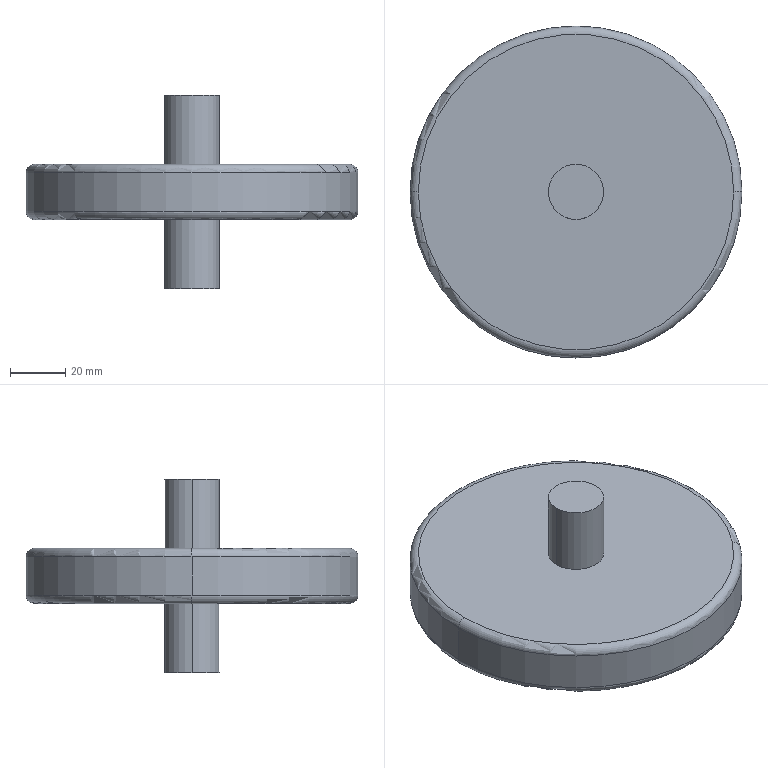Part | SolidWorks | features ICE 2, Extrusion 1, Fillet 1 | 1 solid | 14 faces | box 120 x 120 x 70 mm | volume 240463 mm3 | cylinder 6 | torus 4 | plane 4 | commonest cylinder face diameters 20 x4 120 x2
STEP:
#1=CARTESIAN_POINT('',(10.,0.,45.));
#2=VERTEX_POINT('',#1);
#3=CARTESIAN_POINT('',(-10.,0.,45.));
#4=VERTEX_POINT('',#3);
#5=CARTESIAN_POINT('',(0.,0.,45.));
#6=DIRECTION('',(0.,0.,1.));
#7=DIRECTION('',(1.,0.,0.));
#8=AXIS2_PLACEMENT_3D('',#5,#6,#7);
#9=CIRCLE('',#8,10.);
#10=EDGE_CURVE('',#2,#4,#9,.T.);
#11=ORIENTED_EDGE('',*,*,#10,.F.);
#12=CARTESIAN_POINT('',(10.,0.,20.));
#13=VERTEX_POINT('',#12);
#14=CARTESIAN_POINT('',(10.,0.,45.));
#15=DIRECTION('',(0.,0.,-1.));
#16=VECTOR('',#15,1000.);
#17=LINE('',#14,#16);
#18=EDGE_CURVE('',#2,#13,#17,.T.);
#19=ORIENTED_EDGE('',*,*,#18,.T.);
#20=CARTESIAN_POINT('',(-10.,0.,20.));
#21=VERTEX_POINT('',#20);
#22=CARTESIAN_POINT('',(0.,0.,20.));
#23=DIRECTION('',(0.,0.,1.));
#24=DIRECTION('',(1.,0.,0.));
#25=AXIS2_PLACEMENT_3D('',#22,#23,#24);
#26=CIRCLE('',#25,10.);
#27=EDGE_CURVE('',#13,#21,#26,.T.);
#28=ORIENTED_EDGE('',*,*,#27,.T.);
#29=CARTESIAN_POINT('',(-10.,0.,45.));
#30=DIRECTION('',(0.,0.,-1.));
#31=VECTOR('',#30,1000.);
#32=LINE('',#29,#31);
#33=EDGE_CURVE('',#4,#21,#32,.T.);
#34=ORIENTED_EDGE('',*,*,#33,.F.);
#35=EDGE_LOOP('',(#11,#19,#28,#34));
#36=FACE_OUTER_BOUND('',#35,.T.);
#37=CARTESIAN_POINT('',(0.,0.,45.));
#38=DIRECTION('',(0.,0.,-1.));
#39=DIRECTION('',(-1.,0.,0.));
#40=AXIS2_PLACEMENT_3D('',#37,#38,#39);
#41=CYLINDRICAL_SURFACE('',#40,10.);
#42=ADVANCED_FACE('',(#36),#41,.T.);
#43=CARTESIAN_POINT('',(-10.,0.,-25.));
#44=VERTEX_POINT('',#43);
#45=CARTESIAN_POINT('',(10.,0.,-25.));
#46=VERTEX_POINT('',#45);
#47=CARTESIAN_POINT('',(0.,0.,-25.));
#48=DIRECTION('',(0.,0.,-1.));
#49=DIRECTION('',(-1.,0.,0.));
#50=AXIS2_PLACEMENT_3D('',#47,#48,#49);
#51=CIRCLE('',#50,10.);
#52=EDGE_CURVE('',#44,#46,#51,.T.);
#53=ORIENTED_EDGE('',*,*,#52,.F.);
#54=CARTESIAN_POINT('',(-10.,0.,0.));
#55=VERTEX_POINT('',#54);
#56=CARTESIAN_POINT('',(-10.,0.,-25.));
#57=DIRECTION('',(0.,0.,1.));
#58=VECTOR('',#57,1000.);
#59=LINE('',#56,#58);
#60=EDGE_CURVE('',#44,#55,#59,.T.);
#61=ORIENTED_EDGE('',*,*,#60,.T.);
#62=CARTESIAN_POINT('',(10.,0.,0.));
#63=VERTEX_POINT('',#62);
#64=CARTESIAN_POINT('',(0.,0.,0.));
#65=DIRECTION('',(0.,0.,-1.));
#66=DIRECTION('',(1.,0.,0.));
#67=AXIS2_PLACEMENT_3D('',#64,#65,#66);
#68=CIRCLE('',#67,10.);
#69=EDGE_CURVE('',#55,#63,#68,.T.);
#70=ORIENTED_EDGE('',*,*,#69,.T.);
#71=CARTESIAN_POINT('',(10.,0.,-25.));
#72=DIRECTION('',(0.,0.,1.));
#73=VECTOR('',#72,1000.);
#74=LINE('',#71,#73);
#75=EDGE_CURVE('',#46,#63,#74,.T.);
#76=ORIENTED_EDGE('',*,*,#75,.F.);
#77=EDGE_LOOP('',(#53,#61,#70,#76));
#78=FACE_OUTER_BOUND('',#77,.T.);
#79=CARTESIAN_POINT('',(0.,0.,-25.));
#80=DIRECTION('',(0.,0.,1.));
#81=DIRECTION('',(1.,0.,0.));
#82=AXIS2_PLACEMENT_3D('',#79,#80,#81);
#83=CYLINDRICAL_SURFACE('',#82,10.);
#84=ADVANCED_FACE('',(#78),#83,.T.);
#85=CARTESIAN_POINT('',(-60.,0.,17.));
#86=VERTEX_POINT('',#85);
#87=CARTESIAN_POINT('',(60.,0.,17.));
#88=VERTEX_POINT('',#87);
#89=CARTESIAN_POINT('',(0.,0.,17.));
#90=DIRECTION('',(0.,0.,-1.));
#91=DIRECTION('',(1.,0.,0.));
#92=AXIS2_PLACEMENT_3D('',#89,#90,#91);
#93=CIRCLE('',#92,60.);
#94=EDGE_CURVE('',#86,#88,#93,.T.);
#95=ORIENTED_EDGE('',*,*,#94,.F.);
#96=CARTESIAN_POINT('',(-57.,0.,20.));
#97=VERTEX_POINT('',#96);
#98=CARTESIAN_POINT('',(-57.,0.,17.));
#99=DIRECTION('',(0.,1.,0.));
#100=DIRECTION('',(-1.,0.,0.));
#101=AXIS2_PLACEMENT_3D('',#98,#99,#100);
#102=CIRCLE('',#101,3.);
#103=EDGE_CURVE('',#86,#97,#102,.T.);
#104=ORIENTED_EDGE('',*,*,#103,.T.);
#105=CARTESIAN_POINT('',(57.,0.,20.));
#106=VERTEX_POINT('',#105);
#107=CARTESIAN_POINT('',(0.,0.,20.));
#108=DIRECTION('',(0.,0.,1.));
#109=DIRECTION('',(1.,0.,0.));
#110=AXIS2_PLACEMENT_3D('',#107,#108,#109);
#111=CIRCLE('',#110,57.);
#112=EDGE_CURVE('',#106,#97,#111,.T.);
#113=ORIENTED_EDGE('',*,*,#112,.F.);
#114=CARTESIAN_POINT('',(57.,0.,17.));
#115=DIRECTION('',(0.,-1.,0.));
#116=DIRECTION('',(0.,0.,-1.));
#117=AXIS2_PLACEMENT_3D('',#114,#115,#116);
#118=CIRCLE('',#117,3.);
#119=EDGE_CURVE('',#88,#106,#118,.T.);
#120=ORIENTED_EDGE('',*,*,#119,.F.);
#121=EDGE_LOOP('',(#95,#104,#113,#120));
#122=FACE_OUTER_BOUND('',#121,.T.);
#123=CARTESIAN_POINT('',(0.,0.,17.));
#124=DIRECTION('',(0.,0.,1.));
#125=DIRECTION('',(1.,0.,0.));
#126=AXIS2_PLACEMENT_3D('',#123,#124,#125);
#127=TOROIDAL_SURFACE('',#126,57.,3.);
#128=ADVANCED_FACE('',(#122),#127,.T.);
#129=CARTESIAN_POINT('',(-57.,0.,0.));
#130=VERTEX_POINT('',#129);
#131=CARTESIAN_POINT('',(57.,0.,0.));
#132=VERTEX_POINT('',#131);
#133=CARTESIAN_POINT('',(0.,0.,0.));
#134=DIRECTION('',(0.,0.,-1.));
#135=DIRECTION('',(1.,0.,0.));
#136=AXIS2_PLACEMENT_3D('',#133,#134,#135);
#137=CIRCLE('',#136,57.);
#138=EDGE_CURVE('',#130,#132,#137,.T.);
#139=ORIENTED_EDGE('',*,*,#138,.F.);
#140=CARTESIAN_POINT('',(-60.,0.,3.));
#141=VERTEX_POINT('',#140);
#142=CARTESIAN_POINT('',(-57.,0.,3.));
#143=DIRECTION('',(0.,1.,0.));
#144=DIRECTION('',(-1.,0.,0.));
#145=AXIS2_PLACEMENT_3D('',#142,#143,#144);
#146=CIRCLE('',#145,3.);
#147=EDGE_CURVE('',#130,#141,#146,.T.);
#148=ORIENTED_EDGE('',*,*,#147,.T.);
#149=CARTESIAN_POINT('',(60.,0.,3.));
#150=VERTEX_POINT('',#149);
#151=CARTESIAN_POINT('',(0.,0.,3.));
#152=DIRECTION('',(0.,0.,1.));
#153=DIRECTION('',(1.,0.,0.));
#154=AXIS2_PLACEMENT_3D('',#151,#152,#153);
#155=CIRCLE('',#154,60.);
#156=EDGE_CURVE('',#150,#141,#155,.T.);
#157=ORIENTED_EDGE('',*,*,#156,.F.);
#158=CARTESIAN_POINT('',(57.,0.,3.));
#159=DIRECTION('',(0.,-1.,0.));
#160=DIRECTION('',(0.,0.,-1.));
#161=AXIS2_PLACEMENT_3D('',#158,#159,#160);
#162=CIRCLE('',#161,3.);
#163=EDGE_CURVE('',#132,#150,#162,.T.);
#164=ORIENTED_EDGE('',*,*,#163,.F.);
#165=EDGE_LOOP('',(#139,#148,#157,#164));
#166=FACE_OUTER_BOUND('',#165,.T.);
#167=CARTESIAN_POINT('',(0.,0.,3.));
#168=DIRECTION('',(0.,0.,1.));
#169=DIRECTION('',(1.,0.,0.));
#170=AXIS2_PLACEMENT_3D('',#167,#168,#169);
#171=TOROIDAL_SURFACE('',#170,57.,3.);
#172=ADVANCED_FACE('',(#166),#171,.T.);
#173=ORIENTED_EDGE('',*,*,#94,.T.);
#174=CARTESIAN_POINT('',(60.,0.,20.));
#175=DIRECTION('',(0.,0.,-1.));
#176=VECTOR('',#175,1000.);
#177=LINE('',#174,#176);
#178=EDGE_CURVE('',#88,#150,#177,.T.);
#179=ORIENTED_EDGE('',*,*,#178,.T.);
#180=ORIENTED_EDGE('',*,*,#156,.T.);
#181=CARTESIAN_POINT('',(-60.,0.,20.));
#182=DIRECTION('',(0.,0.,-1.));
#183=VECTOR('',#182,1000.);
#184=LINE('',#181,#183);
#185=EDGE_CURVE('',#86,#141,#184,.T.);
#186=ORIENTED_EDGE('',*,*,#185,.F.);
#187=EDGE_LOOP('',(#173,#179,#180,#186));
#188=FACE_OUTER_BOUND('',#187,.T.);
#189=CARTESIAN_POINT('',(0.,0.,20.));
#190=DIRECTION('',(0.,0.,-1.));
#191=DIRECTION('',(-1.,0.,0.));
#192=AXIS2_PLACEMENT_3D('',#189,#190,#191);
#193=CYLINDRICAL_SURFACE('',#192,60.);
#194=ADVANCED_FACE('',(#188),#193,.T.);
#195=ORIENTED_EDGE('',*,*,#178,.F.);
#196=CARTESIAN_POINT('',(0.,0.,17.));
#197=DIRECTION('',(0.,0.,-1.));
#198=DIRECTION('',(1.,0.,0.));
#199=AXIS2_PLACEMENT_3D('',#196,#197,#198);
#200=CIRCLE('',#199,60.);
#201=EDGE_CURVE('',#88,#86,#200,.T.);
#202=ORIENTED_EDGE('',*,*,#201,.T.);
#203=ORIENTED_EDGE('',*,*,#185,.T.);
#204=CARTESIAN_POINT('',(0.,0.,3.));
#205=DIRECTION('',(0.,0.,1.));
#206=DIRECTION('',(1.,0.,0.));
#207=AXIS2_PLACEMENT_3D('',#204,#205,#206);
#208=CIRCLE('',#207,60.);
#209=EDGE_CURVE('',#141,#150,#208,.T.);
#210=ORIENTED_EDGE('',*,*,#209,.T.);
#211=EDGE_LOOP('',(#195,#202,#203,#210));
#212=FACE_OUTER_BOUND('',#211,.T.);
#213=CARTESIAN_POINT('',(0.,0.,20.));
#214=DIRECTION('',(0.,0.,-1.));
#215=DIRECTION('',(-1.,0.,0.));
#216=AXIS2_PLACEMENT_3D('',#213,#214,#215);
#217=CYLINDRICAL_SURFACE('',#216,60.);
#218=ADVANCED_FACE('',(#212),#217,.T.);
#219=CARTESIAN_POINT('',(0.,0.,20.));
#220=DIRECTION('',(0.,0.,1.));
#221=DIRECTION('',(1.,0.,0.));
#222=AXIS2_PLACEMENT_3D('',#219,#220,#221);
#223=CIRCLE('',#222,10.);
#224=EDGE_CURVE('',#21,#13,#223,.T.);
#225=ORIENTED_EDGE('',*,*,#224,.F.);
#226=ORIENTED_EDGE('',*,*,#27,.F.);
#227=EDGE_LOOP('',(#225,#226));
#228=FACE_BOUND('',#227,.T.);
#229=ORIENTED_EDGE('',*,*,#112,.T.);
#230=CARTESIAN_POINT('',(0.,0.,20.));
#231=DIRECTION('',(0.,0.,1.));
#232=DIRECTION('',(1.,0.,0.));
#233=AXIS2_PLACEMENT_3D('',#230,#231,#232);
#234=CIRCLE('',#233,57.);
#235=EDGE_CURVE('',#97,#106,#234,.T.);
#236=ORIENTED_EDGE('',*,*,#235,.T.);
#237=EDGE_LOOP('',(#229,#236));
#238=FACE_OUTER_BOUND('',#237,.T.);
#239=CARTESIAN_POINT('',(0.,0.,20.));
#240=DIRECTION('',(0.,0.,1.));
#241=DIRECTION('',(1.,0.,0.));
#242=AXIS2_PLACEMENT_3D('',#239,#240,#241);
#243=PLANE('',#242);
#244=ADVANCED_FACE('',(#228,#238),#243,.T.);
#245=CARTESIAN_POINT('',(0.,0.,0.));
#246=DIRECTION('',(0.,0.,-1.));
#247=DIRECTION('',(1.,0.,0.));
#248=AXIS2_PLACEMENT_3D('',#245,#246,#247);
#249=CIRCLE('',#248,10.);
#250=EDGE_CURVE('',#63,#55,#249,.T.);
#251=ORIENTED_EDGE('',*,*,#250,.F.);
#252=ORIENTED_EDGE('',*,*,#69,.F.);
#253=EDGE_LOOP('',(#251,#252));
#254=FACE_BOUND('',#253,.T.);
#255=CARTESIAN_POINT('',(0.,0.,0.));
#256=DIRECTION('',(0.,0.,-1.));
#257=DIRECTION('',(1.,0.,0.));
#258=AXIS2_PLACEMENT_3D('',#255,#256,#257);
#259=CIRCLE('',#258,57.);
#260=EDGE_CURVE('',#132,#130,#259,.T.);
#261=ORIENTED_EDGE('',*,*,#260,.T.);
#262=ORIENTED_EDGE('',*,*,#138,.T.);
#263=EDGE_LOOP('',(#261,#262));
#264=FACE_OUTER_BOUND('',#263,.T.);
#265=CARTESIAN_POINT('',(0.,0.,0.));
#266=DIRECTION('',(0.,0.,1.));
#267=DIRECTION('',(1.,0.,0.));
#268=AXIS2_PLACEMENT_3D('',#265,#266,#267);
#269=PLANE('',#268);
#270=ADVANCED_FACE('',(#254,#264),#269,.F.);
#271=ORIENTED_EDGE('',*,*,#147,.F.);
#272=ORIENTED_EDGE('',*,*,#260,.F.);
#273=ORIENTED_EDGE('',*,*,#163,.T.);
#274=ORIENTED_EDGE('',*,*,#209,.F.);
#275=EDGE_LOOP('',(#271,#272,#273,#274));
#276=FACE_OUTER_BOUND('',#275,.T.);
#277=CARTESIAN_POINT('',(0.,0.,3.));
#278=DIRECTION('',(0.,0.,1.));
#279=DIRECTION('',(1.,0.,0.));
#280=AXIS2_PLACEMENT_3D('',#277,#278,#279);
#281=TOROIDAL_SURFACE('',#280,57.,3.);
#282=ADVANCED_FACE('',(#276),#281,.T.);
#283=ORIENTED_EDGE('',*,*,#103,.F.);
#284=ORIENTED_EDGE('',*,*,#201,.F.);
#285=ORIENTED_EDGE('',*,*,#119,.T.);
#286=ORIENTED_EDGE('',*,*,#235,.F.);
#287=EDGE_LOOP('',(#283,#284,#285,#286));
#288=FACE_OUTER_BOUND('',#287,.T.);
#289=CARTESIAN_POINT('',(0.,0.,17.));
#290=DIRECTION('',(0.,0.,1.));
#291=DIRECTION('',(1.,0.,0.));
#292=AXIS2_PLACEMENT_3D('',#289,#290,#291);
#293=TOROIDAL_SURFACE('',#292,57.,3.);
#294=ADVANCED_FACE('',(#288),#293,.T.);
#295=ORIENTED_EDGE('',*,*,#60,.F.);
#296=CARTESIAN_POINT('',(0.,0.,-25.));
#297=DIRECTION('',(0.,0.,-1.));
#298=DIRECTION('',(-1.,0.,0.));
#299=AXIS2_PLACEMENT_3D('',#296,#297,#298);
#300=CIRCLE('',#299,10.);
#301=EDGE_CURVE('',#46,#44,#300,.T.);
#302=ORIENTED_EDGE('',*,*,#301,.F.);
#303=ORIENTED_EDGE('',*,*,#75,.T.);
#304=ORIENTED_EDGE('',*,*,#250,.T.);
#305=EDGE_LOOP('',(#295,#302,#303,#304));
#306=FACE_OUTER_BOUND('',#305,.T.);
#307=CARTESIAN_POINT('',(0.,0.,-25.));
#308=DIRECTION('',(0.,0.,1.));
#309=DIRECTION('',(1.,0.,0.));
#310=AXIS2_PLACEMENT_3D('',#307,#308,#309);
#311=CYLINDRICAL_SURFACE('',#310,10.);
#312=ADVANCED_FACE('',(#306),#311,.T.);
#313=ORIENTED_EDGE('',*,*,#301,.T.);
#314=ORIENTED_EDGE('',*,*,#52,.T.);
#315=EDGE_LOOP('',(#313,#314));
#316=FACE_OUTER_BOUND('',#315,.T.);
#317=CARTESIAN_POINT('',(0.,0.,-25.));
#318=DIRECTION('',(0.,0.,-1.));
#319=DIRECTION('',(-1.,0.,0.));
#320=AXIS2_PLACEMENT_3D('',#317,#318,#319);
#321=PLANE('',#320);
#322=ADVANCED_FACE('',(#316),#321,.T.);
#323=ORIENTED_EDGE('',*,*,#18,.F.);
#324=CARTESIAN_POINT('',(0.,0.,45.));
#325=DIRECTION('',(0.,0.,1.));
#326=DIRECTION('',(1.,0.,0.));
#327=AXIS2_PLACEMENT_3D('',#324,#325,#326);
#328=CIRCLE('',#327,10.);
#329=EDGE_CURVE('',#4,#2,#328,.T.);
#330=ORIENTED_EDGE('',*,*,#329,.F.);
#331=ORIENTED_EDGE('',*,*,#33,.T.);
#332=ORIENTED_EDGE('',*,*,#224,.T.);
#333=EDGE_LOOP('',(#323,#330,#331,#332));
#334=FACE_OUTER_BOUND('',#333,.T.);
#335=CARTESIAN_POINT('',(0.,0.,45.));
#336=DIRECTION('',(0.,0.,-1.));
#337=DIRECTION('',(-1.,0.,0.));
#338=AXIS2_PLACEMENT_3D('',#335,#336,#337);
#339=CYLINDRICAL_SURFACE('',#338,10.);
#340=ADVANCED_FACE('',(#334),#339,.T.);
#341=ORIENTED_EDGE('',*,*,#329,.T.);
#342=ORIENTED_EDGE('',*,*,#10,.T.);
#343=EDGE_LOOP('',(#341,#342));
#344=FACE_OUTER_BOUND('',#343,.T.);
#345=CARTESIAN_POINT('',(0.,0.,45.));
#346=DIRECTION('',(0.,0.,1.));
#347=DIRECTION('',(1.,0.,0.));
#348=AXIS2_PLACEMENT_3D('',#345,#346,#347);
#349=PLANE('',#348);
#350=ADVANCED_FACE('',(#344),#349,.T.);
#351=CLOSED_SHELL('',(#42,#84,#128,#172,#194,#218,#244,#270,#282,#294,#312,#322,#340,#350));
#352=MANIFOLD_SOLID_BREP('',#351);
#353=CARTESIAN_POINT('',(0.,0.,0.));
#354=DIRECTION('',(0.,0.,1.));
#355=DIRECTION('',(1.,0.,0.));
#356=AXIS2_PLACEMENT_3D('',#353,#354,#355);
#357=(LENGTH_UNIT()NAMED_UNIT(*)SI_UNIT(.MILLI.,.METRE.));
#358=UNCERTAINTY_MEASURE_WITH_UNIT(LENGTH_MEASURE(0.00001),#357,'','');
#359=(NAMED_UNIT(*)PLANE_ANGLE_UNIT()SI_UNIT($,.RADIAN.));
#360=(NAMED_UNIT(*)SI_UNIT($,.STERADIAN.)SOLID_ANGLE_UNIT());
#361=(GEOMETRIC_REPRESENTATION_CONTEXT(3)GLOBAL_UNCERTAINTY_ASSIGNED_CONTEXT((#358))GLOBAL_UNIT_ASSIGNED_CONTEXT((#357,#359,#360))REPRESENTATION_CONTEXT('',''));
#362=ADVANCED_BREP_SHAPE_REPRESENTATION('',(#352,#356),#361);